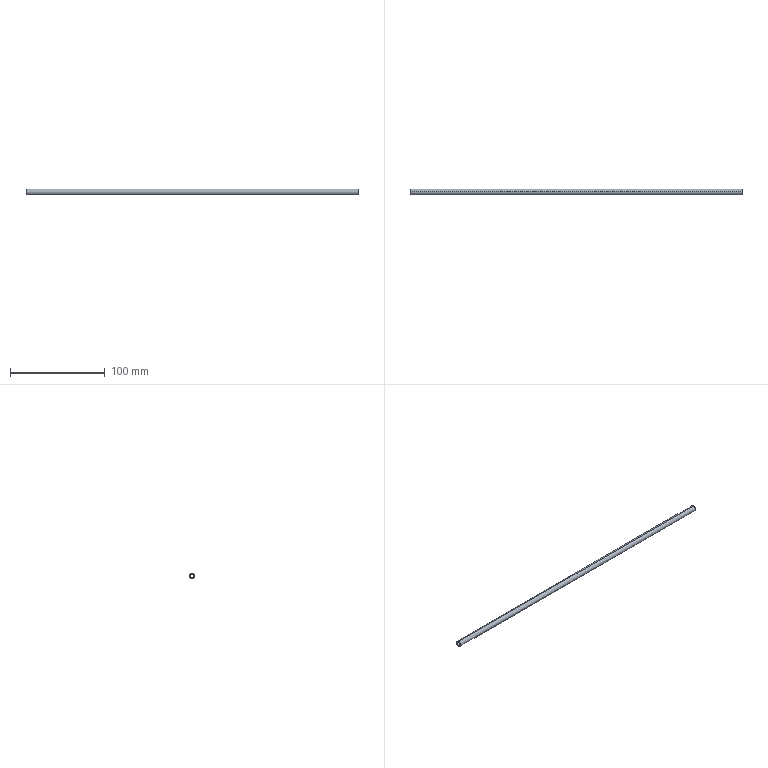Part | SolidWorks | features BaseBody 1 | 1 solid | 6 faces | box 350 x 6 x 6 mm | volume 5498 mm3 | cylinder 4 | plane 2 | commonest cylinder face diameters 4 x2 6 x2
STEP:
#1=CARTESIAN_POINT('',(473.495,13.005,-249.5));
#2=VERTEX_POINT('',#1);
#3=CARTESIAN_POINT('',(473.495,13.005,-245.5));
#4=VERTEX_POINT('',#3);
#5=CARTESIAN_POINT('',(473.495,13.005,-247.5));
#6=DIRECTION('',(1.,0.,0.));
#7=DIRECTION('',(0.,0.,-1.));
#8=AXIS2_PLACEMENT_3D('',#5,#6,#7);
#9=CIRCLE('',#8,2.);
#10=EDGE_CURVE('',#2,#4,#9,.T.);
#11=ORIENTED_EDGE('',*,*,#10,.T.);
#12=CARTESIAN_POINT('',(123.495,13.005,-245.5));
#13=VERTEX_POINT('',#12);
#14=CARTESIAN_POINT('',(123.495,13.005,-245.5));
#15=DIRECTION('',(-1.,0.,0.));
#16=VECTOR('',#15,1000.);
#17=LINE('',#14,#16);
#18=EDGE_CURVE('',#4,#13,#17,.T.);
#19=ORIENTED_EDGE('',*,*,#18,.T.);
#20=CARTESIAN_POINT('',(123.495,13.005,-249.5));
#21=VERTEX_POINT('',#20);
#22=CARTESIAN_POINT('',(123.495,13.005,-247.5));
#23=DIRECTION('',(1.,0.,0.));
#24=DIRECTION('',(0.,0.,-1.));
#25=AXIS2_PLACEMENT_3D('',#22,#23,#24);
#26=CIRCLE('',#25,2.);
#27=EDGE_CURVE('',#21,#13,#26,.T.);
#28=ORIENTED_EDGE('',*,*,#27,.F.);
#29=CARTESIAN_POINT('',(123.495,13.005,-249.5));
#30=DIRECTION('',(-1.,0.,0.));
#31=VECTOR('',#30,1000.);
#32=LINE('',#29,#31);
#33=EDGE_CURVE('',#2,#21,#32,.T.);
#34=ORIENTED_EDGE('',*,*,#33,.F.);
#35=EDGE_LOOP('',(#11,#19,#28,#34));
#36=FACE_OUTER_BOUND('',#35,.T.);
#37=CARTESIAN_POINT('',(123.495,13.005,-247.5));
#38=DIRECTION('',(-1.,0.,0.));
#39=DIRECTION('',(0.,0.,-1.));
#40=AXIS2_PLACEMENT_3D('',#37,#38,#39);
#41=CYLINDRICAL_SURFACE('',#40,2.);
#42=ADVANCED_FACE('',(#36),#41,.F.);
#43=CARTESIAN_POINT('',(473.495,13.005,-244.5));
#44=VERTEX_POINT('',#43);
#45=CARTESIAN_POINT('',(473.495,13.005,-250.5));
#46=VERTEX_POINT('',#45);
#47=CARTESIAN_POINT('',(473.495,13.005,-247.5));
#48=DIRECTION('',(1.,0.,0.));
#49=DIRECTION('',(0.,0.,-1.));
#50=AXIS2_PLACEMENT_3D('',#47,#48,#49);
#51=CIRCLE('',#50,3.);
#52=EDGE_CURVE('',#44,#46,#51,.T.);
#53=ORIENTED_EDGE('',*,*,#52,.F.);
#54=CARTESIAN_POINT('',(123.495,13.005,-244.5));
#55=VERTEX_POINT('',#54);
#56=CARTESIAN_POINT('',(123.495,13.005,-244.5));
#57=DIRECTION('',(-1.,0.,0.));
#58=VECTOR('',#57,1000.);
#59=LINE('',#56,#58);
#60=EDGE_CURVE('',#44,#55,#59,.T.);
#61=ORIENTED_EDGE('',*,*,#60,.T.);
#62=CARTESIAN_POINT('',(123.495,13.005,-250.5));
#63=VERTEX_POINT('',#62);
#64=CARTESIAN_POINT('',(123.495,13.005,-247.5));
#65=DIRECTION('',(1.,0.,0.));
#66=DIRECTION('',(0.,0.,-1.));
#67=AXIS2_PLACEMENT_3D('',#64,#65,#66);
#68=CIRCLE('',#67,3.);
#69=EDGE_CURVE('',#55,#63,#68,.T.);
#70=ORIENTED_EDGE('',*,*,#69,.T.);
#71=CARTESIAN_POINT('',(123.495,13.005,-250.5));
#72=DIRECTION('',(-1.,0.,0.));
#73=VECTOR('',#72,1000.);
#74=LINE('',#71,#73);
#75=EDGE_CURVE('',#46,#63,#74,.T.);
#76=ORIENTED_EDGE('',*,*,#75,.F.);
#77=EDGE_LOOP('',(#53,#61,#70,#76));
#78=FACE_OUTER_BOUND('',#77,.T.);
#79=CARTESIAN_POINT('',(123.495,13.005,-247.5));
#80=DIRECTION('',(-1.,0.,0.));
#81=DIRECTION('',(0.,0.,-1.));
#82=AXIS2_PLACEMENT_3D('',#79,#80,#81);
#83=CYLINDRICAL_SURFACE('',#82,3.);
#84=ADVANCED_FACE('',(#78),#83,.T.);
#85=ORIENTED_EDGE('',*,*,#60,.F.);
#86=CARTESIAN_POINT('',(473.495,13.005,-247.5));
#87=DIRECTION('',(1.,0.,0.));
#88=DIRECTION('',(0.,0.,-1.));
#89=AXIS2_PLACEMENT_3D('',#86,#87,#88);
#90=CIRCLE('',#89,3.);
#91=EDGE_CURVE('',#46,#44,#90,.T.);
#92=ORIENTED_EDGE('',*,*,#91,.F.);
#93=ORIENTED_EDGE('',*,*,#75,.T.);
#94=CARTESIAN_POINT('',(123.495,13.005,-247.5));
#95=DIRECTION('',(1.,0.,0.));
#96=DIRECTION('',(0.,0.,-1.));
#97=AXIS2_PLACEMENT_3D('',#94,#95,#96);
#98=CIRCLE('',#97,3.);
#99=EDGE_CURVE('',#63,#55,#98,.T.);
#100=ORIENTED_EDGE('',*,*,#99,.T.);
#101=EDGE_LOOP('',(#85,#92,#93,#100));
#102=FACE_OUTER_BOUND('',#101,.T.);
#103=CARTESIAN_POINT('',(123.495,13.005,-247.5));
#104=DIRECTION('',(-1.,0.,0.));
#105=DIRECTION('',(0.,0.,-1.));
#106=AXIS2_PLACEMENT_3D('',#103,#104,#105);
#107=CYLINDRICAL_SURFACE('',#106,3.);
#108=ADVANCED_FACE('',(#102),#107,.T.);
#109=ORIENTED_EDGE('',*,*,#10,.F.);
#110=CARTESIAN_POINT('',(473.495,13.005,-247.5));
#111=DIRECTION('',(1.,0.,0.));
#112=DIRECTION('',(0.,0.,-1.));
#113=AXIS2_PLACEMENT_3D('',#110,#111,#112);
#114=CIRCLE('',#113,2.);
#115=EDGE_CURVE('',#4,#2,#114,.T.);
#116=ORIENTED_EDGE('',*,*,#115,.F.);
#117=EDGE_LOOP('',(#109,#116));
#118=FACE_BOUND('',#117,.T.);
#119=ORIENTED_EDGE('',*,*,#91,.T.);
#120=ORIENTED_EDGE('',*,*,#52,.T.);
#121=EDGE_LOOP('',(#119,#120));
#122=FACE_OUTER_BOUND('',#121,.T.);
#123=CARTESIAN_POINT('',(473.495,16.005,-247.5));
#124=DIRECTION('',(1.,0.,0.));
#125=DIRECTION('',(0.,0.,1.));
#126=AXIS2_PLACEMENT_3D('',#123,#124,#125);
#127=PLANE('',#126);
#128=ADVANCED_FACE('',(#118,#122),#127,.T.);
#129=ORIENTED_EDGE('',*,*,#18,.F.);
#130=ORIENTED_EDGE('',*,*,#115,.T.);
#131=ORIENTED_EDGE('',*,*,#33,.T.);
#132=CARTESIAN_POINT('',(123.495,13.005,-247.5));
#133=DIRECTION('',(1.,0.,0.));
#134=DIRECTION('',(0.,0.,-1.));
#135=AXIS2_PLACEMENT_3D('',#132,#133,#134);
#136=CIRCLE('',#135,2.);
#137=EDGE_CURVE('',#13,#21,#136,.T.);
#138=ORIENTED_EDGE('',*,*,#137,.F.);
#139=EDGE_LOOP('',(#129,#130,#131,#138));
#140=FACE_OUTER_BOUND('',#139,.T.);
#141=CARTESIAN_POINT('',(123.495,13.005,-247.5));
#142=DIRECTION('',(-1.,0.,0.));
#143=DIRECTION('',(0.,0.,-1.));
#144=AXIS2_PLACEMENT_3D('',#141,#142,#143);
#145=CYLINDRICAL_SURFACE('',#144,2.);
#146=ADVANCED_FACE('',(#140),#145,.F.);
#147=ORIENTED_EDGE('',*,*,#99,.F.);
#148=ORIENTED_EDGE('',*,*,#69,.F.);
#149=EDGE_LOOP('',(#147,#148));
#150=FACE_OUTER_BOUND('',#149,.T.);
#151=ORIENTED_EDGE('',*,*,#27,.T.);
#152=ORIENTED_EDGE('',*,*,#137,.T.);
#153=EDGE_LOOP('',(#151,#152));
#154=FACE_BOUND('',#153,.T.);
#155=CARTESIAN_POINT('',(123.495,15.005,-247.5));
#156=DIRECTION('',(-1.,0.,0.));
#157=DIRECTION('',(0.,0.,-1.));
#158=AXIS2_PLACEMENT_3D('',#155,#156,#157);
#159=PLANE('',#158);
#160=ADVANCED_FACE('',(#150,#154),#159,.T.);
#161=CLOSED_SHELL('',(#42,#84,#108,#128,#146,#160));
#162=MANIFOLD_SOLID_BREP('',#161);
#163=CARTESIAN_POINT('',(0.,0.,0.));
#164=DIRECTION('',(0.,0.,1.));
#165=DIRECTION('',(1.,0.,0.));
#166=AXIS2_PLACEMENT_3D('',#163,#164,#165);
#167=(LENGTH_UNIT()NAMED_UNIT(*)SI_UNIT(.MILLI.,.METRE.));
#168=UNCERTAINTY_MEASURE_WITH_UNIT(LENGTH_MEASURE(0.00001),#167,'','');
#169=(NAMED_UNIT(*)PLANE_ANGLE_UNIT()SI_UNIT($,.RADIAN.));
#170=(NAMED_UNIT(*)SI_UNIT($,.STERADIAN.)SOLID_ANGLE_UNIT());
#171=(GEOMETRIC_REPRESENTATION_CONTEXT(3)GLOBAL_UNCERTAINTY_ASSIGNED_CONTEXT((#168))GLOBAL_UNIT_ASSIGNED_CONTEXT((#167,#169,#170))REPRESENTATION_CONTEXT('',''));
#172=ADVANCED_BREP_SHAPE_REPRESENTATION('',(#162,#166),#171);